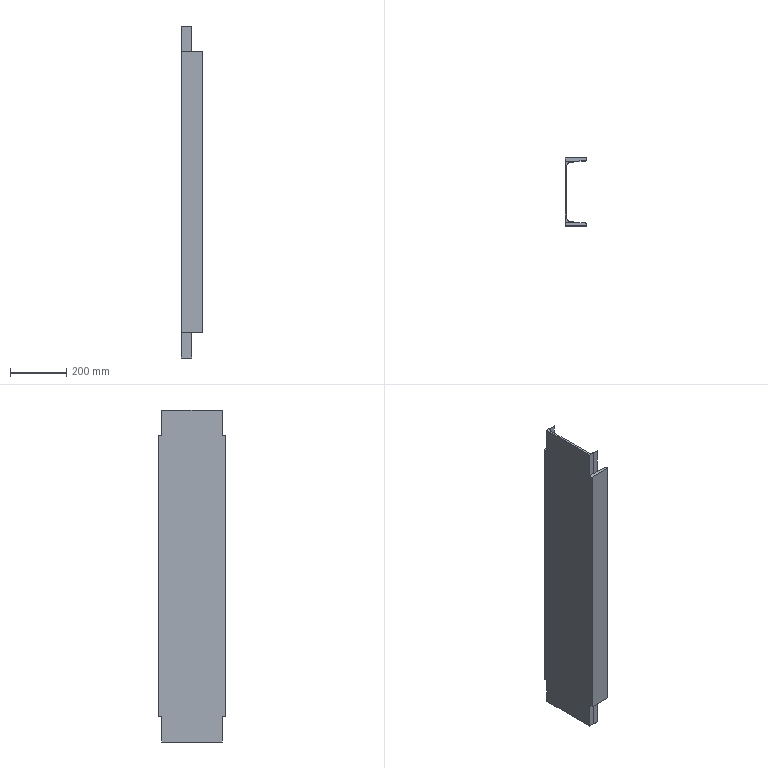Part | NX | features BREP 1, DATUM_CSYS 1, SKETCH 1 | 1 solid | 22 faces | box 78 x 240 x 1180 mm | volume 3661713 mm3 | plane 18 | cylinder 4 | commonest cylinder face diameters 12 x2 24 x2
STEP:
#1=CARTESIAN_POINT('',(78.,116.95,500.));
#2=VERTEX_POINT('',#1);
#3=CARTESIAN_POINT('',(78.,116.95,-500.));
#4=VERTEX_POINT('',#3);
#5=CARTESIAN_POINT('',(78.,116.95,590.));
#6=DIRECTION('',(0.,0.,-1.));
#7=VECTOR('',#6,1000.);
#8=LINE('',#5,#7);
#9=EDGE_CURVE('',#2,#4,#8,.T.);
#10=ORIENTED_EDGE('',*,*,#9,.F.);
#11=CARTESIAN_POINT('',(72.,110.95,500.));
#12=VERTEX_POINT('',#11);
#13=CARTESIAN_POINT('',(72.,116.95,500.));
#14=DIRECTION('',(0.,0.,-1.));
#15=DIRECTION('',(-1.,0.,0.));
#16=AXIS2_PLACEMENT_3D('',#13,#14,#15);
#17=CIRCLE('',#16,6.);
#18=EDGE_CURVE('',#2,#12,#17,.T.);
#19=ORIENTED_EDGE('',*,*,#18,.T.);
#20=CARTESIAN_POINT('',(72.,110.95,-500.));
#21=VERTEX_POINT('',#20);
#22=CARTESIAN_POINT('',(72.,110.95,590.));
#23=DIRECTION('',(0.,0.,-1.));
#24=VECTOR('',#23,1000.);
#25=LINE('',#22,#24);
#26=EDGE_CURVE('',#12,#21,#25,.T.);
#27=ORIENTED_EDGE('',*,*,#26,.T.);
#28=CARTESIAN_POINT('',(72.,116.95,-500.));
#29=DIRECTION('',(0.,0.,1.));
#30=DIRECTION('',(1.,0.,0.));
#31=AXIS2_PLACEMENT_3D('',#28,#29,#30);
#32=CIRCLE('',#31,6.);
#33=EDGE_CURVE('',#21,#4,#32,.T.);
#34=ORIENTED_EDGE('',*,*,#33,.T.);
#35=EDGE_LOOP('',(#10,#19,#27,#34));
#36=FACE_BOUND('',#35,.T.);
#37=CARTESIAN_POINT('',(72.,116.95,590.));
#38=DIRECTION('',(0.,0.,-1.));
#39=DIRECTION('',(1.,0.,0.));
#40=AXIS2_PLACEMENT_3D('',#37,#38,#39);
#41=CYLINDRICAL_SURFACE('',#40,6.);
#42=ADVANCED_FACE('',(#36),#41,.T.);
#43=CARTESIAN_POINT('',(78.,120.,500.));
#44=VERTEX_POINT('',#43);
#45=CARTESIAN_POINT('',(78.,120.,-500.));
#46=VERTEX_POINT('',#45);
#47=CARTESIAN_POINT('',(78.,120.,590.));
#48=DIRECTION('',(0.,0.,-1.));
#49=VECTOR('',#48,1000.);
#50=LINE('',#47,#49);
#51=EDGE_CURVE('',#44,#46,#50,.T.);
#52=ORIENTED_EDGE('',*,*,#51,.F.);
#53=CARTESIAN_POINT('',(78.,120.,500.));
#54=DIRECTION('',(0.,-1.,0.));
#55=VECTOR('',#54,1000.);
#56=LINE('',#53,#55);
#57=EDGE_CURVE('',#44,#2,#56,.T.);
#58=ORIENTED_EDGE('',*,*,#57,.T.);
#59=ORIENTED_EDGE('',*,*,#9,.T.);
#60=CARTESIAN_POINT('',(78.,120.,-500.));
#61=DIRECTION('',(0.,1.,0.));
#62=VECTOR('',#61,1000.);
#63=LINE('',#60,#62);
#64=EDGE_CURVE('',#4,#46,#63,.T.);
#65=ORIENTED_EDGE('',*,*,#64,.T.);
#66=EDGE_LOOP('',(#52,#58,#59,#65));
#67=FACE_BOUND('',#66,.T.);
#68=CARTESIAN_POINT('',(78.,120.,590.));
#69=DIRECTION('',(-1.,0.,0.));
#70=DIRECTION('',(0.,0.,-1.));
#71=AXIS2_PLACEMENT_3D('',#68,#69,#70);
#72=PLANE('',#71);
#73=ADVANCED_FACE('',(#67),#72,.F.);
#74=CARTESIAN_POINT('',(0.,120.,500.));
#75=VERTEX_POINT('',#74);
#76=CARTESIAN_POINT('',(0.,120.,-500.));
#77=VERTEX_POINT('',#76);
#78=CARTESIAN_POINT('',(0.,120.,590.));
#79=DIRECTION('',(0.,0.,-1.));
#80=VECTOR('',#79,1000.);
#81=LINE('',#78,#80);
#82=EDGE_CURVE('',#75,#77,#81,.T.);
#83=ORIENTED_EDGE('',*,*,#82,.F.);
#84=CARTESIAN_POINT('',(78.,120.,500.));
#85=DIRECTION('',(-1.,0.,0.));
#86=VECTOR('',#85,1000.);
#87=LINE('',#84,#86);
#88=EDGE_CURVE('',#44,#75,#87,.T.);
#89=ORIENTED_EDGE('',*,*,#88,.F.);
#90=ORIENTED_EDGE('',*,*,#51,.T.);
#91=CARTESIAN_POINT('',(78.,120.,-500.));
#92=DIRECTION('',(-1.,0.,0.));
#93=VECTOR('',#92,1000.);
#94=LINE('',#91,#93);
#95=EDGE_CURVE('',#46,#77,#94,.T.);
#96=ORIENTED_EDGE('',*,*,#95,.T.);
#97=EDGE_LOOP('',(#83,#89,#90,#96));
#98=FACE_BOUND('',#97,.T.);
#99=CARTESIAN_POINT('',(0.,120.,590.));
#100=DIRECTION('',(0.,-1.,0.));
#101=DIRECTION('',(0.,0.,1.));
#102=AXIS2_PLACEMENT_3D('',#99,#100,#101);
#103=PLANE('',#102);
#104=ADVANCED_FACE('',(#98),#103,.F.);
#105=CARTESIAN_POINT('',(0.,108.,-590.));
#106=VERTEX_POINT('',#105);
#107=CARTESIAN_POINT('',(0.,-108.,-590.));
#108=VERTEX_POINT('',#107);
#109=CARTESIAN_POINT('',(0.,120.,-590.));
#110=DIRECTION('',(0.,-1.,0.));
#111=VECTOR('',#110,1000.);
#112=LINE('',#109,#111);
#113=EDGE_CURVE('',#106,#108,#112,.T.);
#114=ORIENTED_EDGE('',*,*,#113,.T.);
#115=CARTESIAN_POINT('',(0.,-108.,-500.));
#116=VERTEX_POINT('',#115);
#117=CARTESIAN_POINT('',(0.,-108.,-590.));
#118=DIRECTION('',(0.,0.,-1.));
#119=VECTOR('',#118,1000.);
#120=LINE('',#117,#119);
#121=EDGE_CURVE('',#116,#108,#120,.T.);
#122=ORIENTED_EDGE('',*,*,#121,.F.);
#123=CARTESIAN_POINT('',(0.,-120.,-500.));
#124=VERTEX_POINT('',#123);
#125=CARTESIAN_POINT('',(0.,-120.,-500.));
#126=DIRECTION('',(0.,1.,0.));
#127=VECTOR('',#126,1000.);
#128=LINE('',#125,#127);
#129=EDGE_CURVE('',#124,#116,#128,.T.);
#130=ORIENTED_EDGE('',*,*,#129,.F.);
#131=CARTESIAN_POINT('',(0.,-120.,500.));
#132=VERTEX_POINT('',#131);
#133=CARTESIAN_POINT('',(0.,-120.,590.));
#134=DIRECTION('',(0.,0.,-1.));
#135=VECTOR('',#134,1000.);
#136=LINE('',#133,#135);
#137=EDGE_CURVE('',#132,#124,#136,.T.);
#138=ORIENTED_EDGE('',*,*,#137,.F.);
#139=CARTESIAN_POINT('',(0.,-108.,500.));
#140=VERTEX_POINT('',#139);
#141=CARTESIAN_POINT('',(0.,-120.,500.));
#142=DIRECTION('',(0.,-1.,0.));
#143=VECTOR('',#142,1000.);
#144=LINE('',#141,#143);
#145=EDGE_CURVE('',#140,#132,#144,.T.);
#146=ORIENTED_EDGE('',*,*,#145,.F.);
#147=CARTESIAN_POINT('',(0.,-108.,590.));
#148=VERTEX_POINT('',#147);
#149=CARTESIAN_POINT('',(0.,-108.,590.));
#150=DIRECTION('',(0.,0.,-1.));
#151=VECTOR('',#150,1000.);
#152=LINE('',#149,#151);
#153=EDGE_CURVE('',#148,#140,#152,.T.);
#154=ORIENTED_EDGE('',*,*,#153,.F.);
#155=CARTESIAN_POINT('',(0.,108.,590.));
#156=VERTEX_POINT('',#155);
#157=CARTESIAN_POINT('',(0.,120.,590.));
#158=DIRECTION('',(0.,-1.,0.));
#159=VECTOR('',#158,1000.);
#160=LINE('',#157,#159);
#161=EDGE_CURVE('',#156,#148,#160,.T.);
#162=ORIENTED_EDGE('',*,*,#161,.F.);
#163=CARTESIAN_POINT('',(0.,108.,500.));
#164=VERTEX_POINT('',#163);
#165=CARTESIAN_POINT('',(0.,108.,590.));
#166=DIRECTION('',(0.,0.,1.));
#167=VECTOR('',#166,1000.);
#168=LINE('',#165,#167);
#169=EDGE_CURVE('',#164,#156,#168,.T.);
#170=ORIENTED_EDGE('',*,*,#169,.F.);
#171=CARTESIAN_POINT('',(0.,120.,500.));
#172=DIRECTION('',(0.,-1.,0.));
#173=VECTOR('',#172,1000.);
#174=LINE('',#171,#173);
#175=EDGE_CURVE('',#75,#164,#174,.T.);
#176=ORIENTED_EDGE('',*,*,#175,.F.);
#177=ORIENTED_EDGE('',*,*,#82,.T.);
#178=CARTESIAN_POINT('',(0.,108.,-500.));
#179=VERTEX_POINT('',#178);
#180=CARTESIAN_POINT('',(0.,120.,-500.));
#181=DIRECTION('',(0.,1.,0.));
#182=VECTOR('',#181,1000.);
#183=LINE('',#180,#182);
#184=EDGE_CURVE('',#179,#77,#183,.T.);
#185=ORIENTED_EDGE('',*,*,#184,.F.);
#186=CARTESIAN_POINT('',(0.,108.,-590.));
#187=DIRECTION('',(0.,0.,1.));
#188=VECTOR('',#187,1000.);
#189=LINE('',#186,#188);
#190=EDGE_CURVE('',#106,#179,#189,.T.);
#191=ORIENTED_EDGE('',*,*,#190,.F.);
#192=EDGE_LOOP('',(#114,#122,#130,#138,#146,#154,#162,#170,#176,#177,#185,#191));
#193=FACE_BOUND('',#192,.T.);
#194=CARTESIAN_POINT('',(0.,120.,590.));
#195=DIRECTION('',(1.,0.,0.));
#196=DIRECTION('',(0.,0.,1.));
#197=AXIS2_PLACEMENT_3D('',#194,#195,#196);
#198=PLANE('',#197);
#199=ADVANCED_FACE('',(#193),#198,.F.);
#200=ORIENTED_EDGE('',*,*,#137,.T.);
#201=CARTESIAN_POINT('',(78.,-120.,-500.));
#202=VERTEX_POINT('',#201);
#203=CARTESIAN_POINT('',(78.,-120.,-500.));
#204=DIRECTION('',(-1.,0.,0.));
#205=VECTOR('',#204,1000.);
#206=LINE('',#203,#205);
#207=EDGE_CURVE('',#202,#124,#206,.T.);
#208=ORIENTED_EDGE('',*,*,#207,.F.);
#209=CARTESIAN_POINT('',(78.,-120.,500.));
#210=VERTEX_POINT('',#209);
#211=CARTESIAN_POINT('',(78.,-120.,590.));
#212=DIRECTION('',(0.,0.,-1.));
#213=VECTOR('',#212,1000.);
#214=LINE('',#211,#213);
#215=EDGE_CURVE('',#210,#202,#214,.T.);
#216=ORIENTED_EDGE('',*,*,#215,.F.);
#217=CARTESIAN_POINT('',(78.,-120.,500.));
#218=DIRECTION('',(-1.,0.,0.));
#219=VECTOR('',#218,1000.);
#220=LINE('',#217,#219);
#221=EDGE_CURVE('',#210,#132,#220,.T.);
#222=ORIENTED_EDGE('',*,*,#221,.T.);
#223=EDGE_LOOP('',(#200,#208,#216,#222));
#224=FACE_BOUND('',#223,.T.);
#225=CARTESIAN_POINT('',(0.,-120.,590.));
#226=DIRECTION('',(0.,1.,0.));
#227=DIRECTION('',(0.,0.,-1.));
#228=AXIS2_PLACEMENT_3D('',#225,#226,#227);
#229=PLANE('',#228);
#230=ADVANCED_FACE('',(#224),#229,.F.);
#231=ORIENTED_EDGE('',*,*,#215,.T.);
#232=CARTESIAN_POINT('',(78.,-116.95,-500.));
#233=VERTEX_POINT('',#232);
#234=CARTESIAN_POINT('',(78.,-120.,-500.));
#235=DIRECTION('',(0.,1.,0.));
#236=VECTOR('',#235,1000.);
#237=LINE('',#234,#236);
#238=EDGE_CURVE('',#202,#233,#237,.T.);
#239=ORIENTED_EDGE('',*,*,#238,.T.);
#240=CARTESIAN_POINT('',(78.,-116.95,500.));
#241=VERTEX_POINT('',#240);
#242=CARTESIAN_POINT('',(78.,-116.95,590.));
#243=DIRECTION('',(0.,0.,-1.));
#244=VECTOR('',#243,1000.);
#245=LINE('',#242,#244);
#246=EDGE_CURVE('',#241,#233,#245,.T.);
#247=ORIENTED_EDGE('',*,*,#246,.F.);
#248=CARTESIAN_POINT('',(78.,-120.,500.));
#249=DIRECTION('',(0.,-1.,0.));
#250=VECTOR('',#249,1000.);
#251=LINE('',#248,#250);
#252=EDGE_CURVE('',#241,#210,#251,.T.);
#253=ORIENTED_EDGE('',*,*,#252,.T.);
#254=EDGE_LOOP('',(#231,#239,#247,#253));
#255=FACE_BOUND('',#254,.T.);
#256=CARTESIAN_POINT('',(78.,-120.,590.));
#257=DIRECTION('',(-1.,0.,0.));
#258=DIRECTION('',(0.,0.,-1.));
#259=AXIS2_PLACEMENT_3D('',#256,#257,#258);
#260=PLANE('',#259);
#261=ADVANCED_FACE('',(#255),#260,.F.);
#262=ORIENTED_EDGE('',*,*,#246,.T.);
#263=CARTESIAN_POINT('',(72.,-110.95,-500.));
#264=VERTEX_POINT('',#263);
#265=CARTESIAN_POINT('',(72.,-116.95,-500.));
#266=DIRECTION('',(0.,0.,1.));
#267=DIRECTION('',(0.,-1.,0.));
#268=AXIS2_PLACEMENT_3D('',#265,#266,#267);
#269=CIRCLE('',#268,6.);
#270=EDGE_CURVE('',#233,#264,#269,.T.);
#271=ORIENTED_EDGE('',*,*,#270,.T.);
#272=CARTESIAN_POINT('',(72.,-110.95,500.));
#273=VERTEX_POINT('',#272);
#274=CARTESIAN_POINT('',(72.,-110.95,590.));
#275=DIRECTION('',(0.,0.,-1.));
#276=VECTOR('',#275,1000.);
#277=LINE('',#274,#276);
#278=EDGE_CURVE('',#273,#264,#277,.T.);
#279=ORIENTED_EDGE('',*,*,#278,.F.);
#280=CARTESIAN_POINT('',(72.,-116.95,500.));
#281=DIRECTION('',(0.,0.,-1.));
#282=DIRECTION('',(-1.,0.,0.));
#283=AXIS2_PLACEMENT_3D('',#280,#281,#282);
#284=CIRCLE('',#283,6.);
#285=EDGE_CURVE('',#273,#241,#284,.T.);
#286=ORIENTED_EDGE('',*,*,#285,.T.);
#287=EDGE_LOOP('',(#262,#271,#279,#286));
#288=FACE_BOUND('',#287,.T.);
#289=CARTESIAN_POINT('',(72.,-116.95,590.));
#290=DIRECTION('',(0.,0.,-1.));
#291=DIRECTION('',(1.,0.,0.));
#292=AXIS2_PLACEMENT_3D('',#289,#290,#291);
#293=CYLINDRICAL_SURFACE('',#292,6.);
#294=ADVANCED_FACE('',(#288),#293,.T.);
#295=CARTESIAN_POINT('',(38.011,-108.,-500.));
#296=VERTEX_POINT('',#295);
#297=CARTESIAN_POINT('',(72.,-110.95,-500.));
#298=DIRECTION('',(-0.9963,0.08647,0.));
#299=VECTOR('',#298,1000.);
#300=LINE('',#297,#299);
#301=EDGE_CURVE('',#264,#296,#300,.T.);
#302=ORIENTED_EDGE('',*,*,#301,.T.);
#303=CARTESIAN_POINT('',(38.011,-108.,-590.));
#304=VERTEX_POINT('',#303);
#305=CARTESIAN_POINT('',(38.011,-108.,590.));
#306=DIRECTION('',(0.,0.,-1.));
#307=VECTOR('',#306,1000.);
#308=LINE('',#305,#307);
#309=EDGE_CURVE('',#296,#304,#308,.T.);
#310=ORIENTED_EDGE('',*,*,#309,.T.);
#311=CARTESIAN_POINT('',(19.,-106.35,-590.));
#312=VERTEX_POINT('',#311);
#313=CARTESIAN_POINT('',(72.,-110.95,-590.));
#314=DIRECTION('',(-0.9963,0.08647,0.));
#315=VECTOR('',#314,1000.);
#316=LINE('',#313,#315);
#317=EDGE_CURVE('',#304,#312,#316,.T.);
#318=ORIENTED_EDGE('',*,*,#317,.T.);
#319=CARTESIAN_POINT('',(19.,-106.35,590.));
#320=VERTEX_POINT('',#319);
#321=CARTESIAN_POINT('',(19.,-106.35,590.));
#322=DIRECTION('',(0.,0.,-1.));
#323=VECTOR('',#322,1000.);
#324=LINE('',#321,#323);
#325=EDGE_CURVE('',#320,#312,#324,.T.);
#326=ORIENTED_EDGE('',*,*,#325,.F.);
#327=CARTESIAN_POINT('',(38.011,-108.,590.));
#328=VERTEX_POINT('',#327);
#329=CARTESIAN_POINT('',(72.,-110.95,590.));
#330=DIRECTION('',(-0.9963,0.08647,0.));
#331=VECTOR('',#330,1000.);
#332=LINE('',#329,#331);
#333=EDGE_CURVE('',#328,#320,#332,.T.);
#334=ORIENTED_EDGE('',*,*,#333,.F.);
#335=CARTESIAN_POINT('',(38.011,-108.,500.));
#336=VERTEX_POINT('',#335);
#337=CARTESIAN_POINT('',(38.011,-108.,590.));
#338=DIRECTION('',(0.,0.,-1.));
#339=VECTOR('',#338,1000.);
#340=LINE('',#337,#339);
#341=EDGE_CURVE('',#328,#336,#340,.T.);
#342=ORIENTED_EDGE('',*,*,#341,.T.);
#343=CARTESIAN_POINT('',(72.,-110.95,500.));
#344=DIRECTION('',(0.9963,-0.08647,0.));
#345=VECTOR('',#344,1000.);
#346=LINE('',#343,#345);
#347=EDGE_CURVE('',#336,#273,#346,.T.);
#348=ORIENTED_EDGE('',*,*,#347,.T.);
#349=ORIENTED_EDGE('',*,*,#278,.T.);
#350=EDGE_LOOP('',(#302,#310,#318,#326,#334,#342,#348,#349));
#351=FACE_BOUND('',#350,.T.);
#352=CARTESIAN_POINT('',(72.,-110.95,590.));
#353=DIRECTION('',(-0.08647,-0.9963,0.));
#354=DIRECTION('',(-0.9963,0.08647,0.));
#355=AXIS2_PLACEMENT_3D('',#352,#353,#354);
#356=PLANE('',#355);
#357=ADVANCED_FACE('',(#351),#356,.F.);
#358=CARTESIAN_POINT('',(7.,-94.35,-590.));
#359=VERTEX_POINT('',#358);
#360=CARTESIAN_POINT('',(19.,-94.35,-590.));
#361=DIRECTION('',(0.,0.,-1.));
#362=DIRECTION('',(1.,0.,0.));
#363=AXIS2_PLACEMENT_3D('',#360,#361,#362);
#364=CIRCLE('',#363,12.);
#365=EDGE_CURVE('',#312,#359,#364,.T.);
#366=ORIENTED_EDGE('',*,*,#365,.T.);
#367=CARTESIAN_POINT('',(7.,-94.35,590.));
#368=VERTEX_POINT('',#367);
#369=CARTESIAN_POINT('',(7.,-94.35,590.));
#370=DIRECTION('',(0.,0.,-1.));
#371=VECTOR('',#370,1000.);
#372=LINE('',#369,#371);
#373=EDGE_CURVE('',#368,#359,#372,.T.);
#374=ORIENTED_EDGE('',*,*,#373,.F.);
#375=CARTESIAN_POINT('',(19.,-94.35,590.));
#376=DIRECTION('',(0.,0.,-1.));
#377=DIRECTION('',(1.,0.,0.));
#378=AXIS2_PLACEMENT_3D('',#375,#376,#377);
#379=CIRCLE('',#378,12.);
#380=EDGE_CURVE('',#320,#368,#379,.T.);
#381=ORIENTED_EDGE('',*,*,#380,.F.);
#382=ORIENTED_EDGE('',*,*,#325,.T.);
#383=EDGE_LOOP('',(#366,#374,#381,#382));
#384=FACE_BOUND('',#383,.T.);
#385=CARTESIAN_POINT('',(19.,-94.35,590.));
#386=DIRECTION('',(0.,0.,-1.));
#387=DIRECTION('',(1.,0.,0.));
#388=AXIS2_PLACEMENT_3D('',#385,#386,#387);
#389=CYLINDRICAL_SURFACE('',#388,12.);
#390=ADVANCED_FACE('',(#384),#389,.F.);
#391=CARTESIAN_POINT('',(7.,94.35,-590.));
#392=VERTEX_POINT('',#391);
#393=CARTESIAN_POINT('',(7.,-94.35,-590.));
#394=DIRECTION('',(0.,1.,0.));
#395=VECTOR('',#394,1000.);
#396=LINE('',#393,#395);
#397=EDGE_CURVE('',#359,#392,#396,.T.);
#398=ORIENTED_EDGE('',*,*,#397,.T.);
#399=CARTESIAN_POINT('',(7.,94.35,590.));
#400=VERTEX_POINT('',#399);
#401=CARTESIAN_POINT('',(7.,94.35,590.));
#402=DIRECTION('',(0.,0.,-1.));
#403=VECTOR('',#402,1000.);
#404=LINE('',#401,#403);
#405=EDGE_CURVE('',#400,#392,#404,.T.);
#406=ORIENTED_EDGE('',*,*,#405,.F.);
#407=CARTESIAN_POINT('',(7.,-94.35,590.));
#408=DIRECTION('',(0.,1.,0.));
#409=VECTOR('',#408,1000.);
#410=LINE('',#407,#409);
#411=EDGE_CURVE('',#368,#400,#410,.T.);
#412=ORIENTED_EDGE('',*,*,#411,.F.);
#413=ORIENTED_EDGE('',*,*,#373,.T.);
#414=EDGE_LOOP('',(#398,#406,#412,#413));
#415=FACE_BOUND('',#414,.T.);
#416=CARTESIAN_POINT('',(7.,-94.35,590.));
#417=DIRECTION('',(-1.,0.,0.));
#418=DIRECTION('',(0.,0.,-1.));
#419=AXIS2_PLACEMENT_3D('',#416,#417,#418);
#420=PLANE('',#419);
#421=ADVANCED_FACE('',(#415),#420,.F.);
#422=CARTESIAN_POINT('',(19.,106.35,-590.));
#423=VERTEX_POINT('',#422);
#424=CARTESIAN_POINT('',(19.,94.35,-590.));
#425=DIRECTION('',(0.,0.,-1.));
#426=DIRECTION('',(-1.,0.,0.));
#427=AXIS2_PLACEMENT_3D('',#424,#425,#426);
#428=CIRCLE('',#427,12.);
#429=EDGE_CURVE('',#392,#423,#428,.T.);
#430=ORIENTED_EDGE('',*,*,#429,.T.);
#431=CARTESIAN_POINT('',(19.,106.35,590.));
#432=VERTEX_POINT('',#431);
#433=CARTESIAN_POINT('',(19.,106.35,590.));
#434=DIRECTION('',(0.,0.,-1.));
#435=VECTOR('',#434,1000.);
#436=LINE('',#433,#435);
#437=EDGE_CURVE('',#432,#423,#436,.T.);
#438=ORIENTED_EDGE('',*,*,#437,.F.);
#439=CARTESIAN_POINT('',(19.,94.35,590.));
#440=DIRECTION('',(0.,0.,-1.));
#441=DIRECTION('',(-1.,0.,0.));
#442=AXIS2_PLACEMENT_3D('',#439,#440,#441);
#443=CIRCLE('',#442,12.);
#444=EDGE_CURVE('',#400,#432,#443,.T.);
#445=ORIENTED_EDGE('',*,*,#444,.F.);
#446=ORIENTED_EDGE('',*,*,#405,.T.);
#447=EDGE_LOOP('',(#430,#438,#445,#446));
#448=FACE_BOUND('',#447,.T.);
#449=CARTESIAN_POINT('',(19.,94.35,590.));
#450=DIRECTION('',(0.,0.,-1.));
#451=DIRECTION('',(1.,0.,0.));
#452=AXIS2_PLACEMENT_3D('',#449,#450,#451);
#453=CYLINDRICAL_SURFACE('',#452,12.);
#454=ADVANCED_FACE('',(#448),#453,.F.);
#455=CARTESIAN_POINT('',(38.011,108.,500.));
#456=VERTEX_POINT('',#455);
#457=CARTESIAN_POINT('',(72.,110.95,500.));
#458=DIRECTION('',(-0.9963,-0.08647,0.));
#459=VECTOR('',#458,1000.);
#460=LINE('',#457,#459);
#461=EDGE_CURVE('',#12,#456,#460,.T.);
#462=ORIENTED_EDGE('',*,*,#461,.T.);
#463=CARTESIAN_POINT('',(38.011,108.,590.));
#464=VERTEX_POINT('',#463);
#465=CARTESIAN_POINT('',(38.011,108.,590.));
#466=DIRECTION('',(0.,0.,1.));
#467=VECTOR('',#466,1000.);
#468=LINE('',#465,#467);
#469=EDGE_CURVE('',#456,#464,#468,.T.);
#470=ORIENTED_EDGE('',*,*,#469,.T.);
#471=CARTESIAN_POINT('',(72.,110.95,590.));
#472=DIRECTION('',(0.9963,0.08647,0.));
#473=VECTOR('',#472,1000.);
#474=LINE('',#471,#473);
#475=EDGE_CURVE('',#432,#464,#474,.T.);
#476=ORIENTED_EDGE('',*,*,#475,.F.);
#477=ORIENTED_EDGE('',*,*,#437,.T.);
#478=CARTESIAN_POINT('',(38.011,108.,-590.));
#479=VERTEX_POINT('',#478);
#480=CARTESIAN_POINT('',(72.,110.95,-590.));
#481=DIRECTION('',(0.9963,0.08647,0.));
#482=VECTOR('',#481,1000.);
#483=LINE('',#480,#482);
#484=EDGE_CURVE('',#423,#479,#483,.T.);
#485=ORIENTED_EDGE('',*,*,#484,.T.);
#486=CARTESIAN_POINT('',(38.011,108.,-500.));
#487=VERTEX_POINT('',#486);
#488=CARTESIAN_POINT('',(38.011,108.,590.));
#489=DIRECTION('',(0.,0.,1.));
#490=VECTOR('',#489,1000.);
#491=LINE('',#488,#490);
#492=EDGE_CURVE('',#479,#487,#491,.T.);
#493=ORIENTED_EDGE('',*,*,#492,.T.);
#494=CARTESIAN_POINT('',(72.,110.95,-500.));
#495=DIRECTION('',(0.9963,0.08647,0.));
#496=VECTOR('',#495,1000.);
#497=LINE('',#494,#496);
#498=EDGE_CURVE('',#487,#21,#497,.T.);
#499=ORIENTED_EDGE('',*,*,#498,.T.);
#500=ORIENTED_EDGE('',*,*,#26,.F.);
#501=EDGE_LOOP('',(#462,#470,#476,#477,#485,#493,#499,#500));
#502=FACE_BOUND('',#501,.T.);
#503=CARTESIAN_POINT('',(72.,110.95,590.));
#504=DIRECTION('',(-0.08647,0.9963,0.));
#505=DIRECTION('',(0.9963,0.08647,0.));
#506=AXIS2_PLACEMENT_3D('',#503,#504,#505);
#507=PLANE('',#506);
#508=ADVANCED_FACE('',(#502),#507,.F.);
#509=ORIENTED_EDGE('',*,*,#161,.T.);
#510=CARTESIAN_POINT('',(72.,-108.,590.));
#511=DIRECTION('',(1.,0.,0.));
#512=VECTOR('',#511,1000.);
#513=LINE('',#510,#512);
#514=EDGE_CURVE('',#148,#328,#513,.T.);
#515=ORIENTED_EDGE('',*,*,#514,.T.);
#516=ORIENTED_EDGE('',*,*,#333,.T.);
#517=ORIENTED_EDGE('',*,*,#380,.T.);
#518=ORIENTED_EDGE('',*,*,#411,.T.);
#519=ORIENTED_EDGE('',*,*,#444,.T.);
#520=ORIENTED_EDGE('',*,*,#475,.T.);
#521=CARTESIAN_POINT('',(72.,108.,590.));
#522=DIRECTION('',(-1.,0.,0.));
#523=VECTOR('',#522,1000.);
#524=LINE('',#521,#523);
#525=EDGE_CURVE('',#464,#156,#524,.T.);
#526=ORIENTED_EDGE('',*,*,#525,.T.);
#527=EDGE_LOOP('',(#509,#515,#516,#517,#518,#519,#520,#526));
#528=FACE_BOUND('',#527,.T.);
#529=CARTESIAN_POINT('',(72.,116.95,590.));
#530=DIRECTION('',(0.,0.,-1.));
#531=DIRECTION('',(1.,0.,0.));
#532=AXIS2_PLACEMENT_3D('',#529,#530,#531);
#533=PLANE('',#532);
#534=ADVANCED_FACE('',(#528),#533,.F.);
#535=CARTESIAN_POINT('',(72.,-108.,-590.));
#536=DIRECTION('',(1.,0.,0.));
#537=VECTOR('',#536,1000.);
#538=LINE('',#535,#537);
#539=EDGE_CURVE('',#108,#304,#538,.T.);
#540=ORIENTED_EDGE('',*,*,#539,.F.);
#541=ORIENTED_EDGE('',*,*,#113,.F.);
#542=CARTESIAN_POINT('',(72.,108.,-590.));
#543=DIRECTION('',(-1.,0.,0.));
#544=VECTOR('',#543,1000.);
#545=LINE('',#542,#544);
#546=EDGE_CURVE('',#479,#106,#545,.T.);
#547=ORIENTED_EDGE('',*,*,#546,.F.);
#548=ORIENTED_EDGE('',*,*,#484,.F.);
#549=ORIENTED_EDGE('',*,*,#429,.F.);
#550=ORIENTED_EDGE('',*,*,#397,.F.);
#551=ORIENTED_EDGE('',*,*,#365,.F.);
#552=ORIENTED_EDGE('',*,*,#317,.F.);
#553=EDGE_LOOP('',(#540,#541,#547,#548,#549,#550,#551,#552));
#554=FACE_BOUND('',#553,.T.);
#555=CARTESIAN_POINT('',(72.,116.95,-590.));
#556=DIRECTION('',(0.,0.,-1.));
#557=DIRECTION('',(1.,0.,0.));
#558=AXIS2_PLACEMENT_3D('',#555,#556,#557);
#559=PLANE('',#558);
#560=ADVANCED_FACE('',(#554),#559,.T.);
#561=ORIENTED_EDGE('',*,*,#498,.F.);
#562=CARTESIAN_POINT('',(78.,108.,-500.));
#563=DIRECTION('',(-1.,0.,0.));
#564=VECTOR('',#563,1000.);
#565=LINE('',#562,#564);
#566=EDGE_CURVE('',#487,#179,#565,.T.);
#567=ORIENTED_EDGE('',*,*,#566,.T.);
#568=ORIENTED_EDGE('',*,*,#184,.T.);
#569=ORIENTED_EDGE('',*,*,#95,.F.);
#570=ORIENTED_EDGE('',*,*,#64,.F.);
#571=ORIENTED_EDGE('',*,*,#33,.F.);
#572=EDGE_LOOP('',(#561,#567,#568,#569,#570,#571));
#573=FACE_BOUND('',#572,.T.);
#574=CARTESIAN_POINT('',(78.,120.,-500.));
#575=DIRECTION('',(0.,0.,1.));
#576=DIRECTION('',(-1.,0.,0.));
#577=AXIS2_PLACEMENT_3D('',#574,#575,#576);
#578=PLANE('',#577);
#579=ADVANCED_FACE('',(#573),#578,.F.);
#580=ORIENTED_EDGE('',*,*,#546,.T.);
#581=ORIENTED_EDGE('',*,*,#190,.T.);
#582=ORIENTED_EDGE('',*,*,#566,.F.);
#583=ORIENTED_EDGE('',*,*,#492,.F.);
#584=EDGE_LOOP('',(#580,#581,#582,#583));
#585=FACE_BOUND('',#584,.T.);
#586=CARTESIAN_POINT('',(78.,108.,-590.));
#587=DIRECTION('',(0.,-1.,0.));
#588=DIRECTION('',(0.,0.,1.));
#589=AXIS2_PLACEMENT_3D('',#586,#587,#588);
#590=PLANE('',#589);
#591=ADVANCED_FACE('',(#585),#590,.F.);
#592=ORIENTED_EDGE('',*,*,#57,.F.);
#593=ORIENTED_EDGE('',*,*,#88,.T.);
#594=ORIENTED_EDGE('',*,*,#175,.T.);
#595=CARTESIAN_POINT('',(78.,108.,500.));
#596=DIRECTION('',(-1.,0.,0.));
#597=VECTOR('',#596,1000.);
#598=LINE('',#595,#597);
#599=EDGE_CURVE('',#456,#164,#598,.T.);
#600=ORIENTED_EDGE('',*,*,#599,.F.);
#601=ORIENTED_EDGE('',*,*,#461,.F.);
#602=ORIENTED_EDGE('',*,*,#18,.F.);
#603=EDGE_LOOP('',(#592,#593,#594,#600,#601,#602));
#604=FACE_BOUND('',#603,.T.);
#605=CARTESIAN_POINT('',(78.,120.,500.));
#606=DIRECTION('',(0.,0.,-1.));
#607=DIRECTION('',(1.,0.,0.));
#608=AXIS2_PLACEMENT_3D('',#605,#606,#607);
#609=PLANE('',#608);
#610=ADVANCED_FACE('',(#604),#609,.F.);
#611=ORIENTED_EDGE('',*,*,#599,.T.);
#612=ORIENTED_EDGE('',*,*,#169,.T.);
#613=ORIENTED_EDGE('',*,*,#525,.F.);
#614=ORIENTED_EDGE('',*,*,#469,.F.);
#615=EDGE_LOOP('',(#611,#612,#613,#614));
#616=FACE_BOUND('',#615,.T.);
#617=CARTESIAN_POINT('',(78.,108.,590.));
#618=DIRECTION('',(0.,-1.,0.));
#619=DIRECTION('',(0.,0.,1.));
#620=AXIS2_PLACEMENT_3D('',#617,#618,#619);
#621=PLANE('',#620);
#622=ADVANCED_FACE('',(#616),#621,.F.);
#623=ORIENTED_EDGE('',*,*,#347,.F.);
#624=CARTESIAN_POINT('',(78.,-108.,500.));
#625=DIRECTION('',(-1.,0.,0.));
#626=VECTOR('',#625,1000.);
#627=LINE('',#624,#626);
#628=EDGE_CURVE('',#336,#140,#627,.T.);
#629=ORIENTED_EDGE('',*,*,#628,.T.);
#630=ORIENTED_EDGE('',*,*,#145,.T.);
#631=ORIENTED_EDGE('',*,*,#221,.F.);
#632=ORIENTED_EDGE('',*,*,#252,.F.);
#633=ORIENTED_EDGE('',*,*,#285,.F.);
#634=EDGE_LOOP('',(#623,#629,#630,#631,#632,#633));
#635=FACE_BOUND('',#634,.T.);
#636=CARTESIAN_POINT('',(78.,-120.,500.));
#637=DIRECTION('',(0.,0.,-1.));
#638=DIRECTION('',(1.,0.,0.));
#639=AXIS2_PLACEMENT_3D('',#636,#637,#638);
#640=PLANE('',#639);
#641=ADVANCED_FACE('',(#635),#640,.F.);
#642=ORIENTED_EDGE('',*,*,#514,.F.);
#643=ORIENTED_EDGE('',*,*,#153,.T.);
#644=ORIENTED_EDGE('',*,*,#628,.F.);
#645=ORIENTED_EDGE('',*,*,#341,.F.);
#646=EDGE_LOOP('',(#642,#643,#644,#645));
#647=FACE_BOUND('',#646,.T.);
#648=CARTESIAN_POINT('',(78.,-108.,590.));
#649=DIRECTION('',(0.,1.,0.));
#650=DIRECTION('',(0.,0.,-1.));
#651=AXIS2_PLACEMENT_3D('',#648,#649,#650);
#652=PLANE('',#651);
#653=ADVANCED_FACE('',(#647),#652,.F.);
#654=ORIENTED_EDGE('',*,*,#238,.F.);
#655=ORIENTED_EDGE('',*,*,#207,.T.);
#656=ORIENTED_EDGE('',*,*,#129,.T.);
#657=CARTESIAN_POINT('',(78.,-108.,-500.));
#658=DIRECTION('',(-1.,0.,0.));
#659=VECTOR('',#658,1000.);
#660=LINE('',#657,#659);
#661=EDGE_CURVE('',#296,#116,#660,.T.);
#662=ORIENTED_EDGE('',*,*,#661,.F.);
#663=ORIENTED_EDGE('',*,*,#301,.F.);
#664=ORIENTED_EDGE('',*,*,#270,.F.);
#665=EDGE_LOOP('',(#654,#655,#656,#662,#663,#664));
#666=FACE_BOUND('',#665,.T.);
#667=CARTESIAN_POINT('',(78.,-120.,-500.));
#668=DIRECTION('',(0.,0.,1.));
#669=DIRECTION('',(0.,1.,0.));
#670=AXIS2_PLACEMENT_3D('',#667,#668,#669);
#671=PLANE('',#670);
#672=ADVANCED_FACE('',(#666),#671,.F.);
#673=ORIENTED_EDGE('',*,*,#661,.T.);
#674=ORIENTED_EDGE('',*,*,#121,.T.);
#675=ORIENTED_EDGE('',*,*,#539,.T.);
#676=ORIENTED_EDGE('',*,*,#309,.F.);
#677=EDGE_LOOP('',(#673,#674,#675,#676));
#678=FACE_BOUND('',#677,.T.);
#679=CARTESIAN_POINT('',(78.,-108.,-590.));
#680=DIRECTION('',(0.,1.,0.));
#681=DIRECTION('',(0.,0.,-1.));
#682=AXIS2_PLACEMENT_3D('',#679,#680,#681);
#683=PLANE('',#682);
#684=ADVANCED_FACE('',(#678),#683,.F.);
#685=CLOSED_SHELL('',(#42,#73,#104,#199,#230,#261,#294,#357,#390,#421,#454,#508,#534,#560,#579,#591,#610,#622,#641,#653,#672,#684));
#686=MANIFOLD_SOLID_BREP('',#685);
#687=(LENGTH_UNIT()NAMED_UNIT(*)SI_UNIT(.MILLI.,.METRE.));
#688=UNCERTAINTY_MEASURE_WITH_UNIT(LENGTH_MEASURE(0.00001),#687,'','');
#689=(NAMED_UNIT(*)PLANE_ANGLE_UNIT()SI_UNIT($,.RADIAN.));
#690=(NAMED_UNIT(*)SI_UNIT($,.STERADIAN.)SOLID_ANGLE_UNIT());
#691=(GEOMETRIC_REPRESENTATION_CONTEXT(3)GLOBAL_UNCERTAINTY_ASSIGNED_CONTEXT((#688))GLOBAL_UNIT_ASSIGNED_CONTEXT((#687,#689,#690))REPRESENTATION_CONTEXT('',''));
#692=ADVANCED_BREP_SHAPE_REPRESENTATION('',(#686),#691);